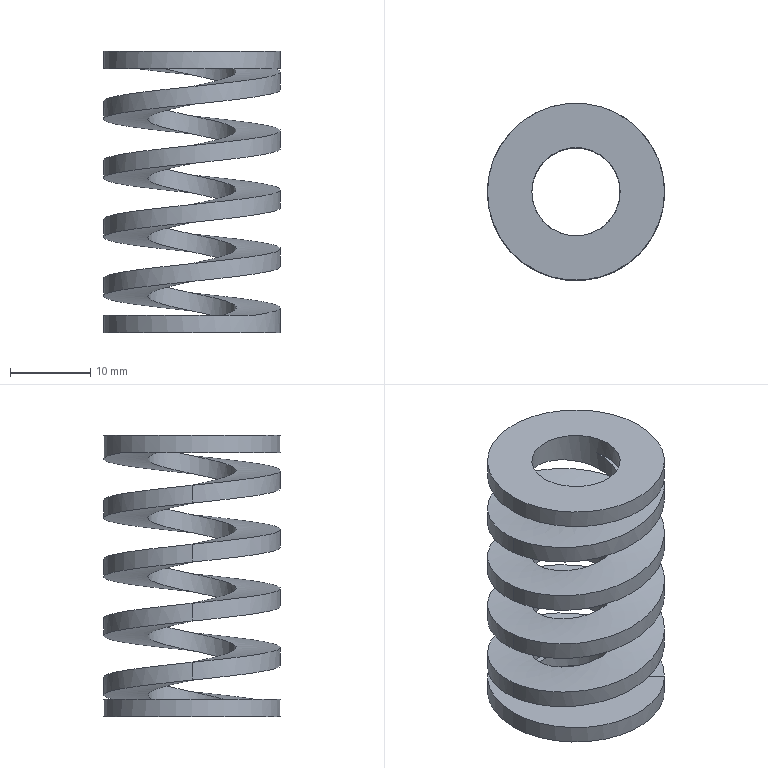Part | STEP file | 1 solid | 123 faces | box 22 x 22 x 35 mm | volume 3894 mm3 | plane 60 | other 51 | cylinder 10 | spline 2 | commonest cylinder face diameters 11 x5 22 x5